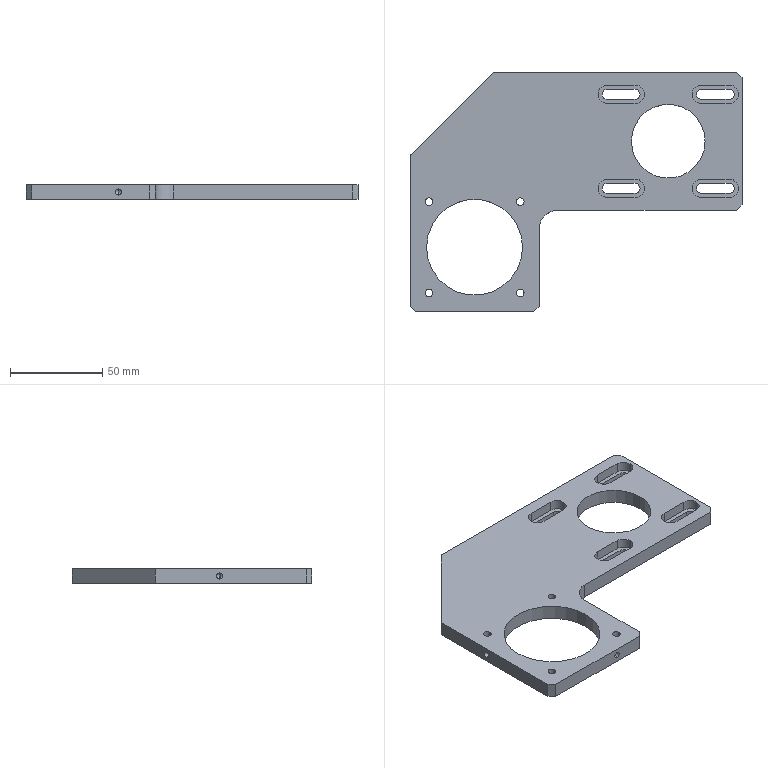Part | SolidWorks | features HoleWzd 7, ICE 7, Chamfer 2, Extrusion 1, Fillet 1, LPattern 1 | 1 solid | 86 faces | box 180 x 130 x 8 mm | volume 96811 mm3 | cylinder 45 | plane 33 | cone 8 | commonest cylinder face diameters 5.5 x12 10 x12 3.3 x8 4.2 x8 40 x2 52 x2